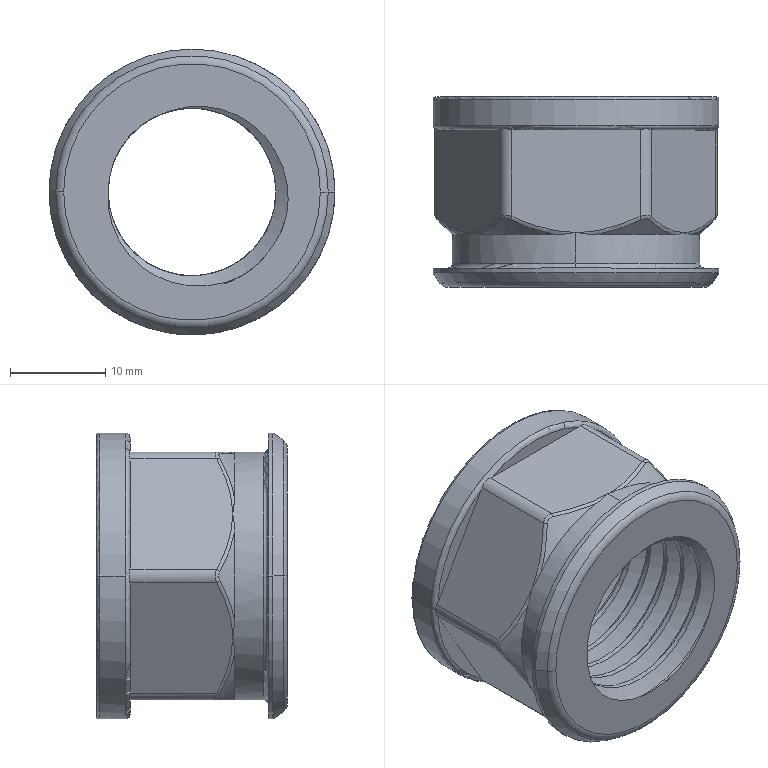Part | STEP file | ZXW722-L-22 | 1 solid | 105 faces | box 30 x 20 x 30 mm | volume 5724 mm3 | spline 33 | cylinder 28 | plane 17 | torus 16 | cone 11 | commonest cylinder face diameters 17.6 x10 2.729 x6 30 x4 21 x2 23 x2 26 x2